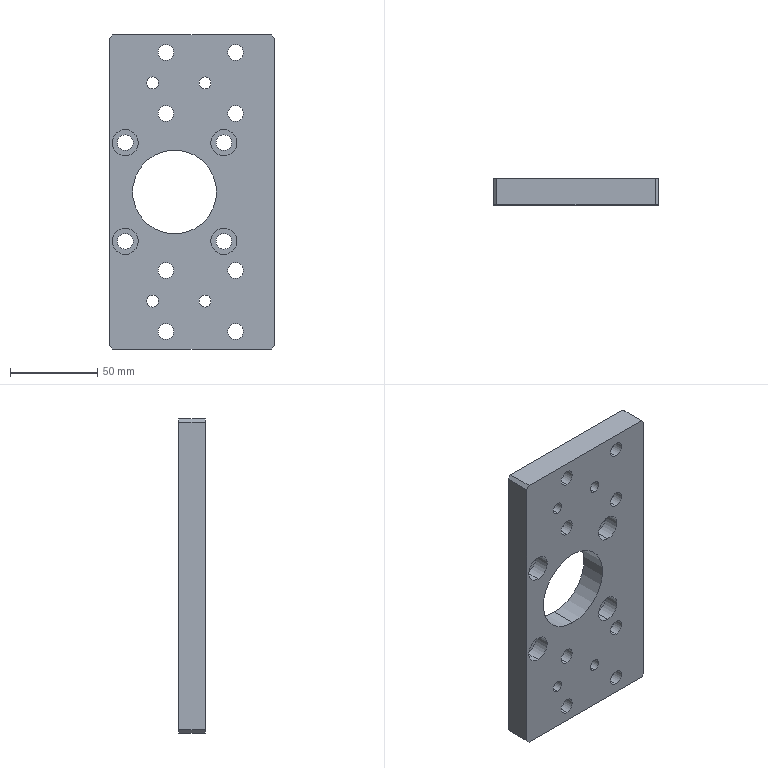Part | STEP file | Cylinder fixing plate | 1 solid | 80 faces | box 95 x 15 x 180 mm | volume 203392 mm3 | cylinder 58 | plane 22 | commonest cylinder face diameters 9 x24 15 x24 6.8 x8 48 x2